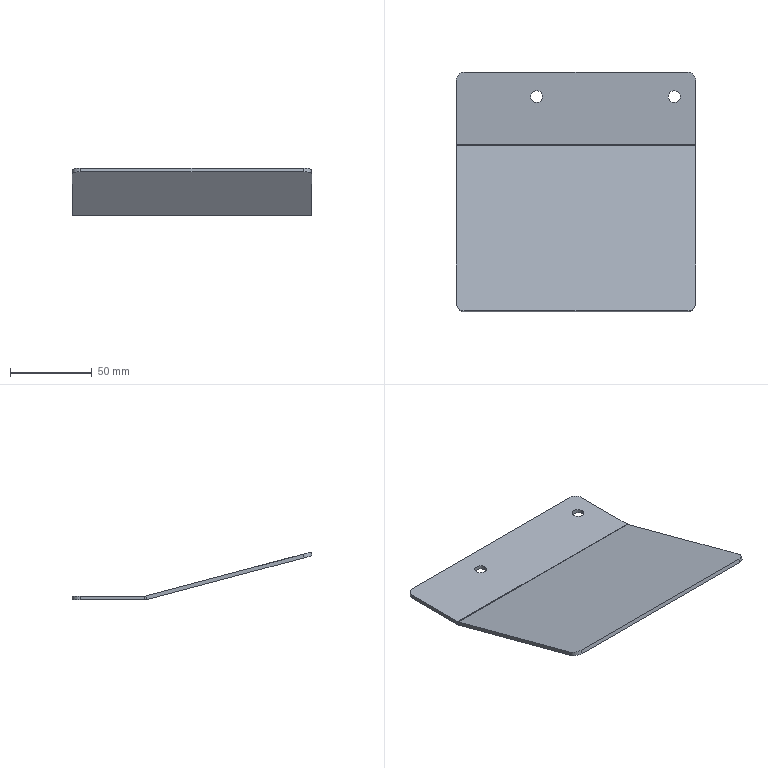Part | SolidWorks | features Fillet 1, FlatPattern 1, ICE 1, SMBaseFlange 1, SheetMetal 1 | 1 solid | 22 faces | box 146 x 146.5 x 29.223 mm | volume 50041 mm3 | plane 12 | cylinder 10 | commonest cylinder face diameters 7.2 x4 10 x4 5 x1 9.6 x1
STEP:
#1=CARTESIAN_POINT('',(56.4,-15.,0.));
#2=VERTEX_POINT('',#1);
#3=CARTESIAN_POINT('',(63.6,-15.,0.));
#4=VERTEX_POINT('',#3);
#5=CARTESIAN_POINT('',(60.,-15.,0.));
#6=DIRECTION('',(0.,0.,1.));
#7=DIRECTION('',(-1.,0.,0.));
#8=AXIS2_PLACEMENT_3D('',#5,#6,#7);
#9=CIRCLE('',#8,3.6);
#10=EDGE_CURVE('',#2,#4,#9,.T.);
#11=ORIENTED_EDGE('',*,*,#10,.F.);
#12=CARTESIAN_POINT('',(56.4,-15.,2.3));
#13=VERTEX_POINT('',#12);
#14=CARTESIAN_POINT('',(56.4,-15.,-0.001));
#15=DIRECTION('',(0.,0.,1.));
#16=VECTOR('',#15,1000.);
#17=LINE('',#14,#16);
#18=EDGE_CURVE('',#2,#13,#17,.T.);
#19=ORIENTED_EDGE('',*,*,#18,.T.);
#20=CARTESIAN_POINT('',(63.6,-15.,2.3));
#21=VERTEX_POINT('',#20);
#22=CARTESIAN_POINT('',(60.,-15.,2.3));
#23=DIRECTION('',(0.,0.,1.));
#24=DIRECTION('',(1.,0.,0.));
#25=AXIS2_PLACEMENT_3D('',#22,#23,#24);
#26=CIRCLE('',#25,3.6);
#27=EDGE_CURVE('',#13,#21,#26,.T.);
#28=ORIENTED_EDGE('',*,*,#27,.T.);
#29=CARTESIAN_POINT('',(63.6,-15.,-0.001));
#30=DIRECTION('',(0.,0.,1.));
#31=VECTOR('',#30,1000.);
#32=LINE('',#29,#31);
#33=EDGE_CURVE('',#4,#21,#32,.T.);
#34=ORIENTED_EDGE('',*,*,#33,.F.);
#35=EDGE_LOOP('',(#11,#19,#28,#34));
#36=FACE_OUTER_BOUND('',#35,.T.);
#37=CARTESIAN_POINT('',(60.,-15.,-0.001));
#38=DIRECTION('',(0.,0.,1.));
#39=DIRECTION('',(1.,0.,0.));
#40=AXIS2_PLACEMENT_3D('',#37,#38,#39);
#41=CYLINDRICAL_SURFACE('',#40,3.6);
#42=ADVANCED_FACE('',(#36),#41,.F.);
#43=CARTESIAN_POINT('',(-27.6,-15.,0.));
#44=VERTEX_POINT('',#43);
#45=CARTESIAN_POINT('',(-20.4,-15.,0.));
#46=VERTEX_POINT('',#45);
#47=CARTESIAN_POINT('',(-24.,-15.,0.));
#48=DIRECTION('',(0.,0.,1.));
#49=DIRECTION('',(-1.,0.,0.));
#50=AXIS2_PLACEMENT_3D('',#47,#48,#49);
#51=CIRCLE('',#50,3.6);
#52=EDGE_CURVE('',#44,#46,#51,.T.);
#53=ORIENTED_EDGE('',*,*,#52,.F.);
#54=CARTESIAN_POINT('',(-27.6,-15.,2.3));
#55=VERTEX_POINT('',#54);
#56=CARTESIAN_POINT('',(-27.6,-15.,-0.001));
#57=DIRECTION('',(0.,0.,1.));
#58=VECTOR('',#57,1000.);
#59=LINE('',#56,#58);
#60=EDGE_CURVE('',#44,#55,#59,.T.);
#61=ORIENTED_EDGE('',*,*,#60,.T.);
#62=CARTESIAN_POINT('',(-20.4,-15.,2.3));
#63=VERTEX_POINT('',#62);
#64=CARTESIAN_POINT('',(-24.,-15.,2.3));
#65=DIRECTION('',(0.,0.,1.));
#66=DIRECTION('',(1.,0.,0.));
#67=AXIS2_PLACEMENT_3D('',#64,#65,#66);
#68=CIRCLE('',#67,3.6);
#69=EDGE_CURVE('',#55,#63,#68,.T.);
#70=ORIENTED_EDGE('',*,*,#69,.T.);
#71=CARTESIAN_POINT('',(-20.4,-15.,-0.001));
#72=DIRECTION('',(0.,0.,1.));
#73=VECTOR('',#72,1000.);
#74=LINE('',#71,#73);
#75=EDGE_CURVE('',#46,#63,#74,.T.);
#76=ORIENTED_EDGE('',*,*,#75,.F.);
#77=EDGE_LOOP('',(#53,#61,#70,#76));
#78=FACE_OUTER_BOUND('',#77,.T.);
#79=CARTESIAN_POINT('',(-24.,-15.,-0.001));
#80=DIRECTION('',(0.,0.,1.));
#81=DIRECTION('',(1.,0.,0.));
#82=AXIS2_PLACEMENT_3D('',#79,#80,#81);
#83=CYLINDRICAL_SURFACE('',#82,3.6);
#84=ADVANCED_FACE('',(#78),#83,.F.);
#85=CARTESIAN_POINT('',(73.,-45.606,0.1613));
#86=VERTEX_POINT('',#85);
#87=CARTESIAN_POINT('',(73.,-45.015,2.384));
#88=VERTEX_POINT('',#87);
#89=CARTESIAN_POINT('',(73.,-45.606,0.1613));
#90=DIRECTION('',(0.,0.2571,0.9664));
#91=VECTOR('',#90,1000.);
#92=LINE('',#89,#91);
#93=EDGE_CURVE('',#86,#88,#92,.T.);
#94=ORIENTED_EDGE('',*,*,#93,.F.);
#95=CARTESIAN_POINT('',(73.,-44.372,0.));
#96=VERTEX_POINT('',#95);
#97=CARTESIAN_POINT('',(73.,-44.372,4.8));
#98=DIRECTION('',(-1.,0.,0.));
#99=DIRECTION('',(0.,0.,-1.));
#100=AXIS2_PLACEMENT_3D('',#97,#98,#99);
#101=CIRCLE('',#100,4.8);
#102=EDGE_CURVE('',#96,#86,#101,.T.);
#103=ORIENTED_EDGE('',*,*,#102,.F.);
#104=CARTESIAN_POINT('',(73.,-44.372,2.3));
#105=VERTEX_POINT('',#104);
#106=CARTESIAN_POINT('',(73.,-44.372,2.3));
#107=DIRECTION('',(0.,0.,-1.));
#108=VECTOR('',#107,1000.);
#109=LINE('',#106,#108);
#110=EDGE_CURVE('',#105,#96,#109,.T.);
#111=ORIENTED_EDGE('',*,*,#110,.F.);
#112=CARTESIAN_POINT('',(73.,-44.372,4.8));
#113=DIRECTION('',(-1.,0.,0.));
#114=DIRECTION('',(0.,0.,-1.));
#115=AXIS2_PLACEMENT_3D('',#112,#113,#114);
#116=CIRCLE('',#115,2.5);
#117=EDGE_CURVE('',#105,#88,#116,.T.);
#118=ORIENTED_EDGE('',*,*,#117,.T.);
#119=EDGE_LOOP('',(#94,#103,#111,#118));
#120=FACE_OUTER_BOUND('',#119,.T.);
#121=CARTESIAN_POINT('',(73.,-45.606,0.1613));
#122=DIRECTION('',(1.,0.,0.));
#123=DIRECTION('',(0.,0.,-1.));
#124=AXIS2_PLACEMENT_3D('',#121,#122,#123);
#125=PLANE('',#124);
#126=ADVANCED_FACE('',(#120),#125,.T.);
#127=CARTESIAN_POINT('',(73.,-141.077,27.937));
#128=VERTEX_POINT('',#127);
#129=CARTESIAN_POINT('',(73.,-44.409,2.223));
#130=DIRECTION('',(0.,-0.9664,0.2571));
#131=VECTOR('',#130,1000.);
#132=LINE('',#129,#131);
#133=EDGE_CURVE('',#88,#128,#132,.T.);
#134=ORIENTED_EDGE('',*,*,#133,.T.);
#135=CARTESIAN_POINT('',(73.,-141.668,25.715));
#136=VERTEX_POINT('',#135);
#137=CARTESIAN_POINT('',(73.,-141.055,28.019));
#138=DIRECTION('',(0.,-0.2571,-0.9664));
#139=VECTOR('',#138,1000.);
#140=LINE('',#137,#139);
#141=EDGE_CURVE('',#128,#136,#140,.T.);
#142=ORIENTED_EDGE('',*,*,#141,.T.);
#143=CARTESIAN_POINT('',(73.,-45.,0.));
#144=DIRECTION('',(0.,-0.9664,0.2571));
#145=VECTOR('',#144,1000.);
#146=LINE('',#143,#145);
#147=EDGE_CURVE('',#86,#136,#146,.T.);
#148=ORIENTED_EDGE('',*,*,#147,.F.);
#149=ORIENTED_EDGE('',*,*,#93,.T.);
#150=EDGE_LOOP('',(#134,#142,#148,#149));
#151=FACE_OUTER_BOUND('',#150,.T.);
#152=CARTESIAN_POINT('',(73.,-44.372,2.3));
#153=DIRECTION('',(1.,0.,0.));
#154=DIRECTION('',(0.,0.,-1.));
#155=AXIS2_PLACEMENT_3D('',#152,#153,#154);
#156=PLANE('',#155);
#157=ADVANCED_FACE('',(#151),#156,.T.);
#158=CARTESIAN_POINT('',(-73.,-44.372,0.));
#159=VERTEX_POINT('',#158);
#160=CARTESIAN_POINT('',(-73.,-44.372,2.3));
#161=VERTEX_POINT('',#160);
#162=CARTESIAN_POINT('',(-73.,-44.372,0.));
#163=DIRECTION('',(0.,0.,1.));
#164=VECTOR('',#163,1000.);
#165=LINE('',#162,#164);
#166=EDGE_CURVE('',#159,#161,#165,.T.);
#167=ORIENTED_EDGE('',*,*,#166,.F.);
#168=CARTESIAN_POINT('',(-73.,-45.606,0.1613));
#169=VERTEX_POINT('',#168);
#170=CARTESIAN_POINT('',(-73.,-44.372,4.8));
#171=DIRECTION('',(-1.,0.,0.));
#172=DIRECTION('',(0.,0.,-1.));
#173=AXIS2_PLACEMENT_3D('',#170,#171,#172);
#174=CIRCLE('',#173,4.8);
#175=EDGE_CURVE('',#159,#169,#174,.T.);
#176=ORIENTED_EDGE('',*,*,#175,.T.);
#177=CARTESIAN_POINT('',(-73.,-45.015,2.384));
#178=VERTEX_POINT('',#177);
#179=CARTESIAN_POINT('',(-73.,-45.015,2.384));
#180=DIRECTION('',(0.,-0.2571,-0.9664));
#181=VECTOR('',#180,1000.);
#182=LINE('',#179,#181);
#183=EDGE_CURVE('',#178,#169,#182,.T.);
#184=ORIENTED_EDGE('',*,*,#183,.F.);
#185=CARTESIAN_POINT('',(-73.,-44.372,4.8));
#186=DIRECTION('',(-1.,0.,0.));
#187=DIRECTION('',(0.,0.,-1.));
#188=AXIS2_PLACEMENT_3D('',#185,#186,#187);
#189=CIRCLE('',#188,2.5);
#190=EDGE_CURVE('',#161,#178,#189,.T.);
#191=ORIENTED_EDGE('',*,*,#190,.F.);
#192=EDGE_LOOP('',(#167,#176,#184,#191));
#193=FACE_OUTER_BOUND('',#192,.T.);
#194=CARTESIAN_POINT('',(-73.,-44.372,0.));
#195=DIRECTION('',(-1.,0.,0.));
#196=DIRECTION('',(0.,0.,1.));
#197=AXIS2_PLACEMENT_3D('',#194,#195,#196);
#198=PLANE('',#197);
#199=ADVANCED_FACE('',(#193),#198,.T.);
#200=CARTESIAN_POINT('',(-73.,-5.,2.3));
#201=VERTEX_POINT('',#200);
#202=CARTESIAN_POINT('',(-73.,0.,2.3));
#203=DIRECTION('',(0.,-1.,0.));
#204=VECTOR('',#203,1000.);
#205=LINE('',#202,#204);
#206=EDGE_CURVE('',#201,#161,#205,.T.);
#207=ORIENTED_EDGE('',*,*,#206,.F.);
#208=CARTESIAN_POINT('',(-73.,-5.,0.));
#209=VERTEX_POINT('',#208);
#210=CARTESIAN_POINT('',(-73.,-5.,2.384));
#211=DIRECTION('',(0.,0.,-1.));
#212=VECTOR('',#211,1000.);
#213=LINE('',#210,#212);
#214=EDGE_CURVE('',#201,#209,#213,.T.);
#215=ORIENTED_EDGE('',*,*,#214,.T.);
#216=CARTESIAN_POINT('',(-73.,0.,0.));
#217=DIRECTION('',(0.,-1.,0.));
#218=VECTOR('',#217,1000.);
#219=LINE('',#216,#218);
#220=EDGE_CURVE('',#209,#159,#219,.T.);
#221=ORIENTED_EDGE('',*,*,#220,.T.);
#222=ORIENTED_EDGE('',*,*,#166,.T.);
#223=EDGE_LOOP('',(#207,#215,#221,#222));
#224=FACE_OUTER_BOUND('',#223,.T.);
#225=CARTESIAN_POINT('',(-73.,-45.015,2.384));
#226=DIRECTION('',(-1.,0.,0.));
#227=DIRECTION('',(0.,0.,1.));
#228=AXIS2_PLACEMENT_3D('',#225,#226,#227);
#229=PLANE('',#228);
#230=ADVANCED_FACE('',(#224),#229,.T.);
#231=CARTESIAN_POINT('',(-73.,-141.077,27.937));
#232=VERTEX_POINT('',#231);
#233=CARTESIAN_POINT('',(-73.,-44.409,2.223));
#234=DIRECTION('',(0.,-0.9664,0.2571));
#235=VECTOR('',#234,1000.);
#236=LINE('',#233,#235);
#237=EDGE_CURVE('',#178,#232,#236,.T.);
#238=ORIENTED_EDGE('',*,*,#237,.T.);
#239=CARTESIAN_POINT('',(-68.,-145.909,29.223));
#240=VERTEX_POINT('',#239);
#241=CARTESIAN_POINT('',(-68.,-141.077,27.937));
#242=DIRECTION('',(0.,0.2571,0.9664));
#243=DIRECTION('',(0.,0.9664,-0.2571));
#244=AXIS2_PLACEMENT_3D('',#241,#242,#243);
#245=CIRCLE('',#244,5.);
#246=EDGE_CURVE('',#232,#240,#245,.T.);
#247=ORIENTED_EDGE('',*,*,#246,.T.);
#248=CARTESIAN_POINT('',(68.,-145.909,29.223));
#249=VERTEX_POINT('',#248);
#250=CARTESIAN_POINT('',(73.,-145.909,29.223));
#251=DIRECTION('',(-1.,0.,0.));
#252=VECTOR('',#251,1000.);
#253=LINE('',#250,#252);
#254=EDGE_CURVE('',#249,#240,#253,.T.);
#255=ORIENTED_EDGE('',*,*,#254,.F.);
#256=CARTESIAN_POINT('',(68.,-141.077,27.937));
#257=DIRECTION('',(0.,0.2571,0.9664));
#258=DIRECTION('',(0.,0.9664,-0.2571));
#259=AXIS2_PLACEMENT_3D('',#256,#257,#258);
#260=CIRCLE('',#259,5.);
#261=EDGE_CURVE('',#249,#128,#260,.T.);
#262=ORIENTED_EDGE('',*,*,#261,.T.);
#263=ORIENTED_EDGE('',*,*,#133,.F.);
#264=CARTESIAN_POINT('',(73.,-45.015,2.384));
#265=DIRECTION('',(-1.,0.,0.));
#266=VECTOR('',#265,1000.);
#267=LINE('',#264,#266);
#268=EDGE_CURVE('',#88,#178,#267,.T.);
#269=ORIENTED_EDGE('',*,*,#268,.T.);
#270=EDGE_LOOP('',(#238,#247,#255,#262,#263,#269));
#271=FACE_OUTER_BOUND('',#270,.T.);
#272=CARTESIAN_POINT('',(73.,-44.409,2.223));
#273=DIRECTION('',(0.,-0.2571,-0.9664));
#274=DIRECTION('',(0.,0.9664,-0.2571));
#275=AXIS2_PLACEMENT_3D('',#272,#273,#274);
#276=PLANE('',#275);
#277=ADVANCED_FACE('',(#271),#276,.F.);
#278=ORIENTED_EDGE('',*,*,#254,.T.);
#279=CARTESIAN_POINT('',(-68.,-146.5,27.));
#280=VERTEX_POINT('',#279);
#281=CARTESIAN_POINT('',(-68.,-146.5,27.));
#282=DIRECTION('',(0.,-0.2571,-0.9664));
#283=VECTOR('',#282,1000.);
#284=LINE('',#281,#283);
#285=EDGE_CURVE('',#240,#280,#284,.T.);
#286=ORIENTED_EDGE('',*,*,#285,.T.);
#287=CARTESIAN_POINT('',(68.,-146.5,27.));
#288=VERTEX_POINT('',#287);
#289=CARTESIAN_POINT('',(73.,-146.5,27.));
#290=DIRECTION('',(-1.,0.,0.));
#291=VECTOR('',#290,1000.);
#292=LINE('',#289,#291);
#293=EDGE_CURVE('',#288,#280,#292,.T.);
#294=ORIENTED_EDGE('',*,*,#293,.F.);
#295=CARTESIAN_POINT('',(68.,-146.5,27.));
#296=DIRECTION('',(0.,0.2571,0.9664));
#297=VECTOR('',#296,1000.);
#298=LINE('',#295,#297);
#299=EDGE_CURVE('',#288,#249,#298,.T.);
#300=ORIENTED_EDGE('',*,*,#299,.T.);
#301=EDGE_LOOP('',(#278,#286,#294,#300));
#302=FACE_OUTER_BOUND('',#301,.T.);
#303=CARTESIAN_POINT('',(73.,-146.5,27.));
#304=DIRECTION('',(0.,-0.9664,0.2571));
#305=DIRECTION('',(0.,-0.2571,-0.9664));
#306=AXIS2_PLACEMENT_3D('',#303,#304,#305);
#307=PLANE('',#306);
#308=ADVANCED_FACE('',(#302),#307,.T.);
#309=ORIENTED_EDGE('',*,*,#293,.T.);
#310=CARTESIAN_POINT('',(-73.,-141.668,25.715));
#311=VERTEX_POINT('',#310);
#312=CARTESIAN_POINT('',(-68.,-141.668,25.715));
#313=DIRECTION('',(0.,-0.2571,-0.9664));
#314=DIRECTION('',(0.,0.9664,-0.2571));
#315=AXIS2_PLACEMENT_3D('',#312,#313,#314);
#316=CIRCLE('',#315,5.);
#317=EDGE_CURVE('',#280,#311,#316,.T.);
#318=ORIENTED_EDGE('',*,*,#317,.T.);
#319=CARTESIAN_POINT('',(-73.,-45.,0.));
#320=DIRECTION('',(0.,-0.9664,0.2571));
#321=VECTOR('',#320,1000.);
#322=LINE('',#319,#321);
#323=EDGE_CURVE('',#169,#311,#322,.T.);
#324=ORIENTED_EDGE('',*,*,#323,.F.);
#325=CARTESIAN_POINT('',(73.,-45.606,0.1613));
#326=DIRECTION('',(-1.,0.,0.));
#327=VECTOR('',#326,1000.);
#328=LINE('',#325,#327);
#329=EDGE_CURVE('',#86,#169,#328,.T.);
#330=ORIENTED_EDGE('',*,*,#329,.F.);
#331=ORIENTED_EDGE('',*,*,#147,.T.);
#332=CARTESIAN_POINT('',(68.,-141.668,25.715));
#333=DIRECTION('',(0.,-0.2571,-0.9664));
#334=DIRECTION('',(0.,0.9664,-0.2571));
#335=AXIS2_PLACEMENT_3D('',#332,#333,#334);
#336=CIRCLE('',#335,5.);
#337=EDGE_CURVE('',#136,#288,#336,.T.);
#338=ORIENTED_EDGE('',*,*,#337,.T.);
#339=EDGE_LOOP('',(#309,#318,#324,#330,#331,#338));
#340=FACE_OUTER_BOUND('',#339,.T.);
#341=CARTESIAN_POINT('',(73.,-45.,0.));
#342=DIRECTION('',(0.,-0.2571,-0.9664));
#343=DIRECTION('',(0.,0.9664,-0.2571));
#344=AXIS2_PLACEMENT_3D('',#341,#342,#343);
#345=PLANE('',#344);
#346=ADVANCED_FACE('',(#340),#345,.T.);
#347=ORIENTED_EDGE('',*,*,#175,.F.);
#348=CARTESIAN_POINT('',(73.,-44.372,0.));
#349=DIRECTION('',(-1.,0.,0.));
#350=VECTOR('',#349,1000.);
#351=LINE('',#348,#350);
#352=EDGE_CURVE('',#96,#159,#351,.T.);
#353=ORIENTED_EDGE('',*,*,#352,.F.);
#354=ORIENTED_EDGE('',*,*,#102,.T.);
#355=ORIENTED_EDGE('',*,*,#329,.T.);
#356=EDGE_LOOP('',(#347,#353,#354,#355));
#357=FACE_OUTER_BOUND('',#356,.T.);
#358=CARTESIAN_POINT('',(73.,-44.372,4.8));
#359=DIRECTION('',(-1.,0.,0.));
#360=DIRECTION('',(0.,0.,1.));
#361=AXIS2_PLACEMENT_3D('',#358,#359,#360);
#362=CYLINDRICAL_SURFACE('',#361,4.8);
#363=ADVANCED_FACE('',(#357),#362,.T.);
#364=CARTESIAN_POINT('',(60.,-15.,0.));
#365=DIRECTION('',(0.,0.,1.));
#366=DIRECTION('',(-1.,0.,0.));
#367=AXIS2_PLACEMENT_3D('',#364,#365,#366);
#368=CIRCLE('',#367,3.6);
#369=EDGE_CURVE('',#4,#2,#368,.T.);
#370=ORIENTED_EDGE('',*,*,#369,.T.);
#371=ORIENTED_EDGE('',*,*,#10,.T.);
#372=EDGE_LOOP('',(#370,#371));
#373=FACE_BOUND('',#372,.T.);
#374=CARTESIAN_POINT('',(-24.,-15.,0.));
#375=DIRECTION('',(0.,0.,1.));
#376=DIRECTION('',(-1.,0.,0.));
#377=AXIS2_PLACEMENT_3D('',#374,#375,#376);
#378=CIRCLE('',#377,3.6);
#379=EDGE_CURVE('',#46,#44,#378,.T.);
#380=ORIENTED_EDGE('',*,*,#379,.T.);
#381=ORIENTED_EDGE('',*,*,#52,.T.);
#382=EDGE_LOOP('',(#380,#381));
#383=FACE_BOUND('',#382,.T.);
#384=ORIENTED_EDGE('',*,*,#220,.F.);
#385=CARTESIAN_POINT('',(-68.,0.,0.));
#386=VERTEX_POINT('',#385);
#387=CARTESIAN_POINT('',(-68.,-5.,0.));
#388=DIRECTION('',(0.,0.,-1.));
#389=DIRECTION('',(-1.,0.,0.));
#390=AXIS2_PLACEMENT_3D('',#387,#388,#389);
#391=CIRCLE('',#390,5.);
#392=EDGE_CURVE('',#209,#386,#391,.T.);
#393=ORIENTED_EDGE('',*,*,#392,.T.);
#394=CARTESIAN_POINT('',(68.,0.,0.));
#395=VERTEX_POINT('',#394);
#396=CARTESIAN_POINT('',(73.,0.,0.));
#397=DIRECTION('',(-1.,0.,0.));
#398=VECTOR('',#397,1000.);
#399=LINE('',#396,#398);
#400=EDGE_CURVE('',#395,#386,#399,.T.);
#401=ORIENTED_EDGE('',*,*,#400,.F.);
#402=CARTESIAN_POINT('',(73.,-5.,0.));
#403=VERTEX_POINT('',#402);
#404=CARTESIAN_POINT('',(68.,-5.,0.));
#405=DIRECTION('',(0.,0.,-1.));
#406=DIRECTION('',(-1.,0.,0.));
#407=AXIS2_PLACEMENT_3D('',#404,#405,#406);
#408=CIRCLE('',#407,5.);
#409=EDGE_CURVE('',#395,#403,#408,.T.);
#410=ORIENTED_EDGE('',*,*,#409,.T.);
#411=CARTESIAN_POINT('',(73.,0.,0.));
#412=DIRECTION('',(0.,-1.,0.));
#413=VECTOR('',#412,1000.);
#414=LINE('',#411,#413);
#415=EDGE_CURVE('',#403,#96,#414,.T.);
#416=ORIENTED_EDGE('',*,*,#415,.T.);
#417=ORIENTED_EDGE('',*,*,#352,.T.);
#418=EDGE_LOOP('',(#384,#393,#401,#410,#416,#417));
#419=FACE_OUTER_BOUND('',#418,.T.);
#420=CARTESIAN_POINT('',(73.,0.,0.));
#421=DIRECTION('',(0.,0.,-1.));
#422=DIRECTION('',(-1.,0.,0.));
#423=AXIS2_PLACEMENT_3D('',#420,#421,#422);
#424=PLANE('',#423);
#425=ADVANCED_FACE('',(#373,#383,#419),#424,.T.);
#426=ORIENTED_EDGE('',*,*,#400,.T.);
#427=CARTESIAN_POINT('',(-68.,0.,2.3));
#428=VERTEX_POINT('',#427);
#429=CARTESIAN_POINT('',(-68.,0.,2.3));
#430=DIRECTION('',(0.,0.,1.));
#431=VECTOR('',#430,1000.);
#432=LINE('',#429,#431);
#433=EDGE_CURVE('',#386,#428,#432,.T.);
#434=ORIENTED_EDGE('',*,*,#433,.T.);
#435=CARTESIAN_POINT('',(68.,0.,2.3));
#436=VERTEX_POINT('',#435);
#437=CARTESIAN_POINT('',(73.,0.,2.3));
#438=DIRECTION('',(-1.,0.,0.));
#439=VECTOR('',#438,1000.);
#440=LINE('',#437,#439);
#441=EDGE_CURVE('',#436,#428,#440,.T.);
#442=ORIENTED_EDGE('',*,*,#441,.F.);
#443=CARTESIAN_POINT('',(68.,0.,2.3));
#444=DIRECTION('',(0.,0.,-1.));
#445=VECTOR('',#444,1000.);
#446=LINE('',#443,#445);
#447=EDGE_CURVE('',#436,#395,#446,.T.);
#448=ORIENTED_EDGE('',*,*,#447,.T.);
#449=EDGE_LOOP('',(#426,#434,#442,#448));
#450=FACE_OUTER_BOUND('',#449,.T.);
#451=CARTESIAN_POINT('',(73.,0.,2.3));
#452=DIRECTION('',(0.,1.,0.));
#453=DIRECTION('',(0.,0.,1.));
#454=AXIS2_PLACEMENT_3D('',#451,#452,#453);
#455=PLANE('',#454);
#456=ADVANCED_FACE('',(#450),#455,.T.);
#457=CARTESIAN_POINT('',(60.,-15.,2.3));
#458=DIRECTION('',(0.,0.,1.));
#459=DIRECTION('',(1.,0.,0.));
#460=AXIS2_PLACEMENT_3D('',#457,#458,#459);
#461=CIRCLE('',#460,3.6);
#462=EDGE_CURVE('',#21,#13,#461,.T.);
#463=ORIENTED_EDGE('',*,*,#462,.F.);
#464=ORIENTED_EDGE('',*,*,#27,.F.);
#465=EDGE_LOOP('',(#463,#464));
#466=FACE_BOUND('',#465,.T.);
#467=CARTESIAN_POINT('',(-24.,-15.,2.3));
#468=DIRECTION('',(0.,0.,1.));
#469=DIRECTION('',(1.,0.,0.));
#470=AXIS2_PLACEMENT_3D('',#467,#468,#469);
#471=CIRCLE('',#470,3.6);
#472=EDGE_CURVE('',#63,#55,#471,.T.);
#473=ORIENTED_EDGE('',*,*,#472,.F.);
#474=ORIENTED_EDGE('',*,*,#69,.F.);
#475=EDGE_LOOP('',(#473,#474));
#476=FACE_BOUND('',#475,.T.);
#477=ORIENTED_EDGE('',*,*,#441,.T.);
#478=CARTESIAN_POINT('',(-68.,-5.,2.3));
#479=DIRECTION('',(0.,0.,1.));
#480=DIRECTION('',(-1.,0.,0.));
#481=AXIS2_PLACEMENT_3D('',#478,#479,#480);
#482=CIRCLE('',#481,5.);
#483=EDGE_CURVE('',#428,#201,#482,.T.);
#484=ORIENTED_EDGE('',*,*,#483,.T.);
#485=ORIENTED_EDGE('',*,*,#206,.T.);
#486=CARTESIAN_POINT('',(73.,-44.372,2.3));
#487=DIRECTION('',(-1.,0.,0.));
#488=VECTOR('',#487,1000.);
#489=LINE('',#486,#488);
#490=EDGE_CURVE('',#105,#161,#489,.T.);
#491=ORIENTED_EDGE('',*,*,#490,.F.);
#492=CARTESIAN_POINT('',(73.,-5.,2.3));
#493=VERTEX_POINT('',#492);
#494=CARTESIAN_POINT('',(73.,0.,2.3));
#495=DIRECTION('',(0.,-1.,0.));
#496=VECTOR('',#495,1000.);
#497=LINE('',#494,#496);
#498=EDGE_CURVE('',#493,#105,#497,.T.);
#499=ORIENTED_EDGE('',*,*,#498,.F.);
#500=CARTESIAN_POINT('',(68.,-5.,2.3));
#501=DIRECTION('',(0.,0.,1.));
#502=DIRECTION('',(-1.,0.,0.));
#503=AXIS2_PLACEMENT_3D('',#500,#501,#502);
#504=CIRCLE('',#503,5.);
#505=EDGE_CURVE('',#493,#436,#504,.T.);
#506=ORIENTED_EDGE('',*,*,#505,.T.);
#507=EDGE_LOOP('',(#477,#484,#485,#491,#499,#506));
#508=FACE_OUTER_BOUND('',#507,.T.);
#509=CARTESIAN_POINT('',(73.,0.,2.3));
#510=DIRECTION('',(0.,0.,-1.));
#511=DIRECTION('',(-1.,0.,0.));
#512=AXIS2_PLACEMENT_3D('',#509,#510,#511);
#513=PLANE('',#512);
#514=ADVANCED_FACE('',(#466,#476,#508),#513,.F.);
#515=ORIENTED_EDGE('',*,*,#190,.T.);
#516=ORIENTED_EDGE('',*,*,#268,.F.);
#517=ORIENTED_EDGE('',*,*,#117,.F.);
#518=ORIENTED_EDGE('',*,*,#490,.T.);
#519=EDGE_LOOP('',(#515,#516,#517,#518));
#520=FACE_OUTER_BOUND('',#519,.T.);
#521=CARTESIAN_POINT('',(73.,-44.372,4.8));
#522=DIRECTION('',(-1.,0.,0.));
#523=DIRECTION('',(0.,0.,1.));
#524=AXIS2_PLACEMENT_3D('',#521,#522,#523);
#525=CYLINDRICAL_SURFACE('',#524,2.5);
#526=ADVANCED_FACE('',(#520),#525,.F.);
#527=ORIENTED_EDGE('',*,*,#415,.F.);
#528=CARTESIAN_POINT('',(73.,-5.,4.8));
#529=DIRECTION('',(0.,0.,1.));
#530=VECTOR('',#529,1000.);
#531=LINE('',#528,#530);
#532=EDGE_CURVE('',#403,#493,#531,.T.);
#533=ORIENTED_EDGE('',*,*,#532,.T.);
#534=ORIENTED_EDGE('',*,*,#498,.T.);
#535=ORIENTED_EDGE('',*,*,#110,.T.);
#536=EDGE_LOOP('',(#527,#533,#534,#535));
#537=FACE_OUTER_BOUND('',#536,.T.);
#538=CARTESIAN_POINT('',(73.,-44.372,4.8));
#539=DIRECTION('',(1.,0.,0.));
#540=DIRECTION('',(0.,0.,-1.));
#541=AXIS2_PLACEMENT_3D('',#538,#539,#540);
#542=PLANE('',#541);
#543=ADVANCED_FACE('',(#537),#542,.T.);
#544=ORIENTED_EDGE('',*,*,#323,.T.);
#545=CARTESIAN_POINT('',(-73.,-141.077,27.937));
#546=DIRECTION('',(0.,0.2571,0.9664));
#547=VECTOR('',#546,1000.);
#548=LINE('',#545,#547);
#549=EDGE_CURVE('',#311,#232,#548,.T.);
#550=ORIENTED_EDGE('',*,*,#549,.T.);
#551=ORIENTED_EDGE('',*,*,#237,.F.);
#552=ORIENTED_EDGE('',*,*,#183,.T.);
#553=EDGE_LOOP('',(#544,#550,#551,#552));
#554=FACE_OUTER_BOUND('',#553,.T.);
#555=CARTESIAN_POINT('',(-73.,-44.372,4.8));
#556=DIRECTION('',(1.,0.,0.));
#557=DIRECTION('',(0.,0.,-1.));
#558=AXIS2_PLACEMENT_3D('',#555,#556,#557);
#559=PLANE('',#558);
#560=ADVANCED_FACE('',(#554),#559,.F.);
#561=ORIENTED_EDGE('',*,*,#60,.F.);
#562=ORIENTED_EDGE('',*,*,#379,.F.);
#563=ORIENTED_EDGE('',*,*,#75,.T.);
#564=ORIENTED_EDGE('',*,*,#472,.T.);
#565=EDGE_LOOP('',(#561,#562,#563,#564));
#566=FACE_OUTER_BOUND('',#565,.T.);
#567=CARTESIAN_POINT('',(-24.,-15.,-0.001));
#568=DIRECTION('',(0.,0.,1.));
#569=DIRECTION('',(1.,0.,0.));
#570=AXIS2_PLACEMENT_3D('',#567,#568,#569);
#571=CYLINDRICAL_SURFACE('',#570,3.6);
#572=ADVANCED_FACE('',(#566),#571,.F.);
#573=ORIENTED_EDGE('',*,*,#18,.F.);
#574=ORIENTED_EDGE('',*,*,#369,.F.);
#575=ORIENTED_EDGE('',*,*,#33,.T.);
#576=ORIENTED_EDGE('',*,*,#462,.T.);
#577=EDGE_LOOP('',(#573,#574,#575,#576));
#578=FACE_OUTER_BOUND('',#577,.T.);
#579=CARTESIAN_POINT('',(60.,-15.,-0.001));
#580=DIRECTION('',(0.,0.,1.));
#581=DIRECTION('',(1.,0.,0.));
#582=AXIS2_PLACEMENT_3D('',#579,#580,#581);
#583=CYLINDRICAL_SURFACE('',#582,3.6);
#584=ADVANCED_FACE('',(#578),#583,.F.);
#585=ORIENTED_EDGE('',*,*,#317,.F.);
#586=ORIENTED_EDGE('',*,*,#285,.F.);
#587=ORIENTED_EDGE('',*,*,#246,.F.);
#588=ORIENTED_EDGE('',*,*,#549,.F.);
#589=EDGE_LOOP('',(#585,#586,#587,#588));
#590=FACE_OUTER_BOUND('',#589,.T.);
#591=CARTESIAN_POINT('',(-68.,-140.434,30.353));
#592=DIRECTION('',(0.,-0.2571,-0.9664));
#593=DIRECTION('',(0.,0.9664,-0.2571));
#594=AXIS2_PLACEMENT_3D('',#591,#592,#593);
#595=CYLINDRICAL_SURFACE('',#594,5.);
#596=ADVANCED_FACE('',(#590),#595,.T.);
#597=ORIENTED_EDGE('',*,*,#337,.F.);
#598=ORIENTED_EDGE('',*,*,#141,.F.);
#599=ORIENTED_EDGE('',*,*,#261,.F.);
#600=ORIENTED_EDGE('',*,*,#299,.F.);
#601=EDGE_LOOP('',(#597,#598,#599,#600));
#602=FACE_OUTER_BOUND('',#601,.T.);
#603=CARTESIAN_POINT('',(68.,-141.668,25.715));
#604=DIRECTION('',(0.,0.2571,0.9664));
#605=DIRECTION('',(0.,-0.9664,0.2571));
#606=AXIS2_PLACEMENT_3D('',#603,#604,#605);
#607=CYLINDRICAL_SURFACE('',#606,5.);
#608=ADVANCED_FACE('',(#602),#607,.T.);
#609=ORIENTED_EDGE('',*,*,#483,.F.);
#610=ORIENTED_EDGE('',*,*,#433,.F.);
#611=ORIENTED_EDGE('',*,*,#392,.F.);
#612=ORIENTED_EDGE('',*,*,#214,.F.);
#613=EDGE_LOOP('',(#609,#610,#611,#612));
#614=FACE_OUTER_BOUND('',#613,.T.);
#615=CARTESIAN_POINT('',(-68.,-5.,2.384));
#616=DIRECTION('',(0.,0.,-1.));
#617=DIRECTION('',(-1.,0.,0.));
#618=AXIS2_PLACEMENT_3D('',#615,#616,#617);
#619=CYLINDRICAL_SURFACE('',#618,5.);
#620=ADVANCED_FACE('',(#614),#619,.T.);
#621=ORIENTED_EDGE('',*,*,#505,.F.);
#622=ORIENTED_EDGE('',*,*,#532,.F.);
#623=ORIENTED_EDGE('',*,*,#409,.F.);
#624=ORIENTED_EDGE('',*,*,#447,.F.);
#625=EDGE_LOOP('',(#621,#622,#623,#624));
#626=FACE_OUTER_BOUND('',#625,.T.);
#627=CARTESIAN_POINT('',(68.,-5.,2.3));
#628=DIRECTION('',(0.,0.,-1.));
#629=DIRECTION('',(-1.,0.,0.));
#630=AXIS2_PLACEMENT_3D('',#627,#628,#629);
#631=CYLINDRICAL_SURFACE('',#630,5.);
#632=ADVANCED_FACE('',(#626),#631,.T.);
#633=CLOSED_SHELL('',(#42,#84,#126,#157,#199,#230,#277,#308,#346,#363,#425,#456,#514,#526,#543,#560,#572,#584,#596,#608,#620,#632));
#634=MANIFOLD_SOLID_BREP('',#633);
#635=CARTESIAN_POINT('',(0.,0.,0.));
#636=DIRECTION('',(0.,0.,1.));
#637=DIRECTION('',(1.,0.,0.));
#638=AXIS2_PLACEMENT_3D('',#635,#636,#637);
#639=(LENGTH_UNIT()NAMED_UNIT(*)SI_UNIT(.MILLI.,.METRE.));
#640=UNCERTAINTY_MEASURE_WITH_UNIT(LENGTH_MEASURE(0.00001),#639,'','');
#641=(NAMED_UNIT(*)PLANE_ANGLE_UNIT()SI_UNIT($,.RADIAN.));
#642=(NAMED_UNIT(*)SI_UNIT($,.STERADIAN.)SOLID_ANGLE_UNIT());
#643=(GEOMETRIC_REPRESENTATION_CONTEXT(3)GLOBAL_UNCERTAINTY_ASSIGNED_CONTEXT((#640))GLOBAL_UNIT_ASSIGNED_CONTEXT((#639,#641,#642))REPRESENTATION_CONTEXT('',''));
#644=ADVANCED_BREP_SHAPE_REPRESENTATION('',(#634,#638),#643);